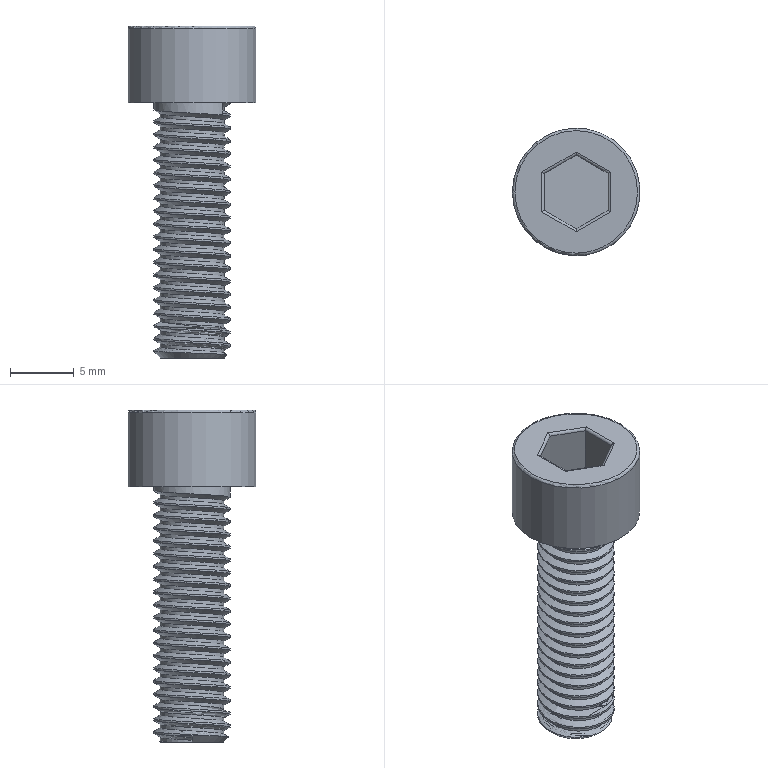Part | STEP file | Tube feed_id1606_x_t | 1 solid | 26 faces | box 10 x 10 x 26 mm | volume 858.061 mm3 | plane 12 | cylinder 9 | spline 3 | torus 1 | cone 1 | commonest cylinder face diameters 0.4 x6 5 x1 6 x1 10 x1